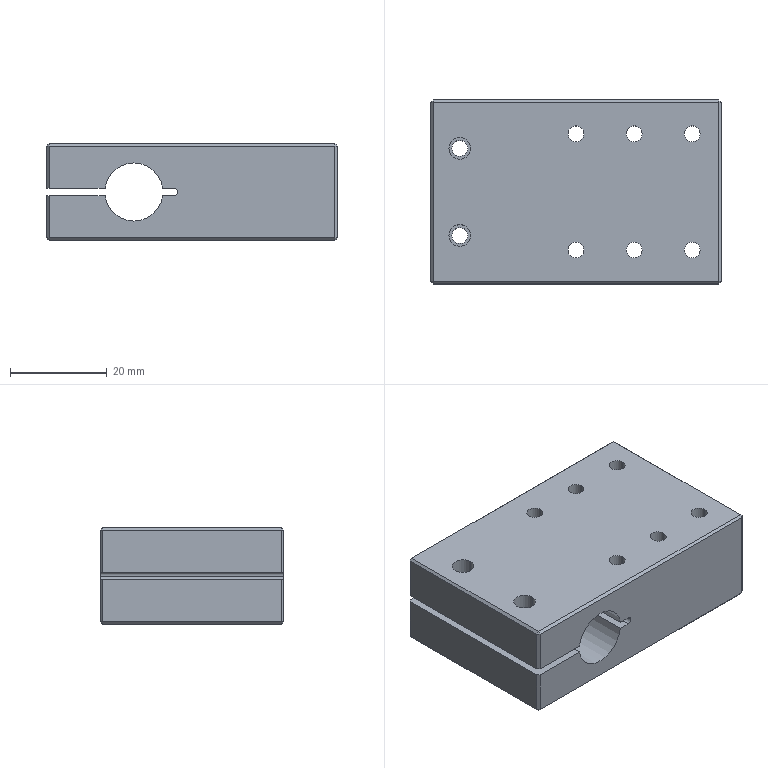Part | STEP file | ND25021-01-JDKM-38-TL | 1 solid | 58 faces | box 60 x 38 x 20 mm | volume 38918 mm3 | plane 33 | cylinder 25 | commonest cylinder face diameters 3.3 x16 4.5 x4 12 x3 1.5 x2